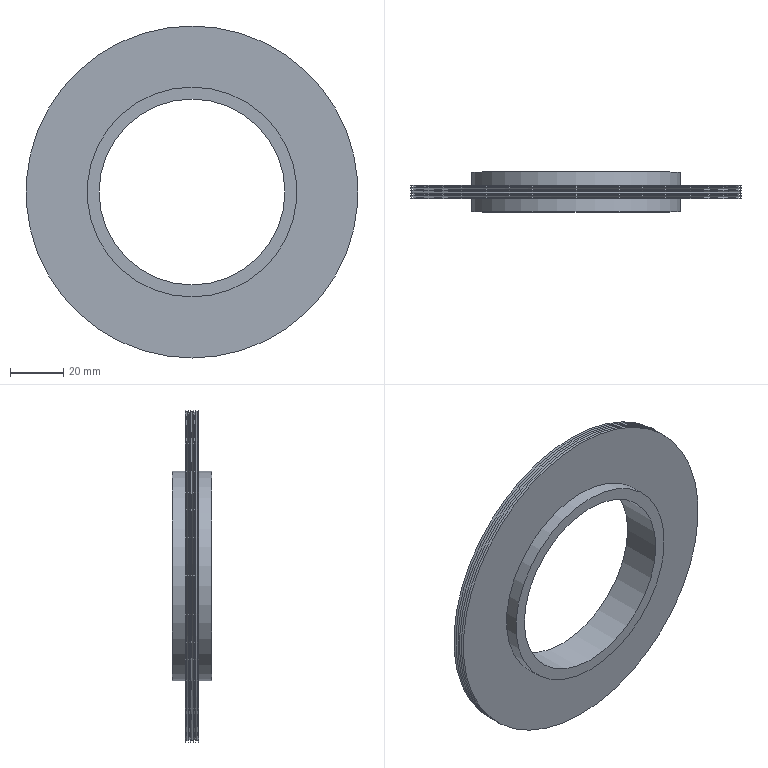Part | NX | 1 solid | 17 faces | box 125 x 15 x 125 mm | volume 51673 mm3 | cone 10 | plane 4 | cylinder 3 | commonest cylinder face diameters 79 x2 70 x1
STEP:
#1=CARTESIAN_POINT('',(0.,18.7,-39.5));
#2=VERTEX_POINT('',#1);
#3=CARTESIAN_POINT('',(0.,18.7,0.));
#4=DIRECTION('',(0.,-1.,0.));
#5=DIRECTION('',(0.,0.,-1.));
#6=AXIS2_PLACEMENT_3D('',#3,#4,#5);
#7=CIRCLE('',#6,39.5);
#8=EDGE_CURVE('',#2,#2,#7,.T.);
#9=ORIENTED_EDGE('',*,*,#8,.T.);
#10=EDGE_LOOP('',(#9));
#11=FACE_BOUND('',#10,.T.);
#12=CARTESIAN_POINT('',(0.,13.7,-39.5));
#13=VERTEX_POINT('',#12);
#14=CARTESIAN_POINT('',(0.,13.7,0.));
#15=DIRECTION('',(0.,-1.,0.));
#16=DIRECTION('',(0.,0.,-1.));
#17=AXIS2_PLACEMENT_3D('',#14,#15,#16);
#18=CIRCLE('',#17,39.5);
#19=EDGE_CURVE('',#13,#13,#18,.T.);
#20=ORIENTED_EDGE('',*,*,#19,.F.);
#21=EDGE_LOOP('',(#20));
#22=FACE_BOUND('',#21,.T.);
#23=CARTESIAN_POINT('',(0.,0.,0.));
#24=DIRECTION('',(0.,-1.,0.));
#25=DIRECTION('',(0.,0.,1.));
#26=AXIS2_PLACEMENT_3D('',#23,#24,#25);
#27=CYLINDRICAL_SURFACE('',#26,39.5);
#28=ADVANCED_FACE('',(#11,#22),#27,.T.);
#29=CARTESIAN_POINT('',(0.,18.7,-35.));
#30=VERTEX_POINT('',#29);
#31=CARTESIAN_POINT('',(0.,18.7,0.));
#32=DIRECTION('',(0.,-1.,0.));
#33=DIRECTION('',(0.,0.,-1.));
#34=AXIS2_PLACEMENT_3D('',#31,#32,#33);
#35=CIRCLE('',#34,35.);
#36=EDGE_CURVE('',#30,#30,#35,.T.);
#37=ORIENTED_EDGE('',*,*,#36,.T.);
#38=EDGE_LOOP('',(#37));
#39=FACE_BOUND('',#38,.T.);
#40=ORIENTED_EDGE('',*,*,#8,.F.);
#41=EDGE_LOOP('',(#40));
#42=FACE_BOUND('',#41,.T.);
#43=CARTESIAN_POINT('',(-39.5,18.7,0.));
#44=DIRECTION('',(0.,1.,0.));
#45=DIRECTION('',(0.,0.,-1.));
#46=AXIS2_PLACEMENT_3D('',#43,#44,#45);
#47=PLANE('',#46);
#48=ADVANCED_FACE('',(#39,#42),#47,.T.);
#49=CARTESIAN_POINT('',(0.,3.7,-35.));
#50=VERTEX_POINT('',#49);
#51=CARTESIAN_POINT('',(0.,3.7,0.));
#52=DIRECTION('',(0.,-1.,0.));
#53=DIRECTION('',(0.,0.,-1.));
#54=AXIS2_PLACEMENT_3D('',#51,#52,#53);
#55=CIRCLE('',#54,35.);
#56=EDGE_CURVE('',#50,#50,#55,.T.);
#57=ORIENTED_EDGE('',*,*,#56,.T.);
#58=EDGE_LOOP('',(#57));
#59=FACE_BOUND('',#58,.T.);
#60=ORIENTED_EDGE('',*,*,#36,.F.);
#61=EDGE_LOOP('',(#60));
#62=FACE_BOUND('',#61,.T.);
#63=CARTESIAN_POINT('',(0.,0.,0.));
#64=DIRECTION('',(0.,-1.,0.));
#65=DIRECTION('',(0.,0.,1.));
#66=AXIS2_PLACEMENT_3D('',#63,#64,#65);
#67=CYLINDRICAL_SURFACE('',#66,35.);
#68=ADVANCED_FACE('',(#59,#62),#67,.F.);
#69=CARTESIAN_POINT('',(0.,3.7,-39.5));
#70=VERTEX_POINT('',#69);
#71=CARTESIAN_POINT('',(0.,3.7,0.));
#72=DIRECTION('',(0.,-1.,0.));
#73=DIRECTION('',(0.,0.,-1.));
#74=AXIS2_PLACEMENT_3D('',#71,#72,#73);
#75=CIRCLE('',#74,39.5);
#76=EDGE_CURVE('',#70,#70,#75,.T.);
#77=ORIENTED_EDGE('',*,*,#76,.T.);
#78=EDGE_LOOP('',(#77));
#79=FACE_BOUND('',#78,.T.);
#80=ORIENTED_EDGE('',*,*,#56,.F.);
#81=EDGE_LOOP('',(#80));
#82=FACE_BOUND('',#81,.T.);
#83=CARTESIAN_POINT('',(-35.,3.7,0.));
#84=DIRECTION('',(0.,-1.,0.));
#85=DIRECTION('',(0.,0.,1.));
#86=AXIS2_PLACEMENT_3D('',#83,#84,#85);
#87=PLANE('',#86);
#88=ADVANCED_FACE('',(#79,#82),#87,.T.);
#89=CARTESIAN_POINT('',(0.,8.7,-39.5));
#90=VERTEX_POINT('',#89);
#91=CARTESIAN_POINT('',(0.,8.7,0.));
#92=DIRECTION('',(0.,-1.,0.));
#93=DIRECTION('',(0.,0.,-1.));
#94=AXIS2_PLACEMENT_3D('',#91,#92,#93);
#95=CIRCLE('',#94,39.5);
#96=EDGE_CURVE('',#90,#90,#95,.T.);
#97=ORIENTED_EDGE('',*,*,#96,.T.);
#98=EDGE_LOOP('',(#97));
#99=FACE_BOUND('',#98,.T.);
#100=ORIENTED_EDGE('',*,*,#76,.F.);
#101=EDGE_LOOP('',(#100));
#102=FACE_BOUND('',#101,.T.);
#103=CARTESIAN_POINT('',(0.,0.,0.));
#104=DIRECTION('',(0.,-1.,0.));
#105=DIRECTION('',(0.,0.,1.));
#106=AXIS2_PLACEMENT_3D('',#103,#104,#105);
#107=CYLINDRICAL_SURFACE('',#106,39.5);
#108=ADVANCED_FACE('',(#99,#102),#107,.T.);
#109=CARTESIAN_POINT('',(0.,8.7,-62.5));
#110=VERTEX_POINT('',#109);
#111=CARTESIAN_POINT('',(0.,8.7,0.));
#112=DIRECTION('',(0.,-1.,0.));
#113=DIRECTION('',(0.,0.,-1.));
#114=AXIS2_PLACEMENT_3D('',#111,#112,#113);
#115=CIRCLE('',#114,62.5);
#116=EDGE_CURVE('',#110,#110,#115,.T.);
#117=ORIENTED_EDGE('',*,*,#116,.T.);
#118=EDGE_LOOP('',(#117));
#119=FACE_BOUND('',#118,.T.);
#120=ORIENTED_EDGE('',*,*,#96,.F.);
#121=EDGE_LOOP('',(#120));
#122=FACE_BOUND('',#121,.T.);
#123=CARTESIAN_POINT('',(-39.5,8.7,0.));
#124=DIRECTION('',(0.,-1.,0.));
#125=DIRECTION('',(0.,0.,1.));
#126=AXIS2_PLACEMENT_3D('',#123,#124,#125);
#127=PLANE('',#126);
#128=ADVANCED_FACE('',(#119,#122),#127,.T.);
#129=CARTESIAN_POINT('',(0.,9.2,-61.5));
#130=VERTEX_POINT('',#129);
#131=CARTESIAN_POINT('',(0.,9.2,0.));
#132=DIRECTION('',(0.,-1.,0.));
#133=DIRECTION('',(0.,0.,-1.));
#134=AXIS2_PLACEMENT_3D('',#131,#132,#133);
#135=CIRCLE('',#134,61.5);
#136=EDGE_CURVE('',#130,#130,#135,.T.);
#137=ORIENTED_EDGE('',*,*,#136,.T.);
#138=EDGE_LOOP('',(#137));
#139=FACE_BOUND('',#138,.T.);
#140=ORIENTED_EDGE('',*,*,#116,.F.);
#141=EDGE_LOOP('',(#140));
#142=FACE_BOUND('',#141,.T.);
#143=CARTESIAN_POINT('',(0.,8.7,0.));
#144=DIRECTION('',(0.,-1.,0.));
#145=DIRECTION('',(0.,0.,1.));
#146=AXIS2_PLACEMENT_3D('',#143,#144,#145);
#147=CONICAL_SURFACE('',#146,62.5,63.435);
#148=ADVANCED_FACE('',(#139,#142),#147,.T.);
#149=CARTESIAN_POINT('',(0.,9.7,-62.5));
#150=VERTEX_POINT('',#149);
#151=CARTESIAN_POINT('',(0.,9.7,0.));
#152=DIRECTION('',(0.,-1.,0.));
#153=DIRECTION('',(0.,0.,-1.));
#154=AXIS2_PLACEMENT_3D('',#151,#152,#153);
#155=CIRCLE('',#154,62.5);
#156=EDGE_CURVE('',#150,#150,#155,.T.);
#157=ORIENTED_EDGE('',*,*,#156,.T.);
#158=EDGE_LOOP('',(#157));
#159=FACE_BOUND('',#158,.T.);
#160=ORIENTED_EDGE('',*,*,#136,.F.);
#161=EDGE_LOOP('',(#160));
#162=FACE_BOUND('',#161,.T.);
#163=CARTESIAN_POINT('',(0.,9.2,0.));
#164=DIRECTION('',(0.,1.,0.));
#165=DIRECTION('',(0.,0.,-1.));
#166=AXIS2_PLACEMENT_3D('',#163,#164,#165);
#167=CONICAL_SURFACE('',#166,61.5,63.435);
#168=ADVANCED_FACE('',(#159,#162),#167,.T.);
#169=CARTESIAN_POINT('',(0.,10.2,-61.5));
#170=VERTEX_POINT('',#169);
#171=CARTESIAN_POINT('',(0.,10.2,0.));
#172=DIRECTION('',(0.,-1.,0.));
#173=DIRECTION('',(0.,0.,-1.));
#174=AXIS2_PLACEMENT_3D('',#171,#172,#173);
#175=CIRCLE('',#174,61.5);
#176=EDGE_CURVE('',#170,#170,#175,.T.);
#177=ORIENTED_EDGE('',*,*,#176,.T.);
#178=EDGE_LOOP('',(#177));
#179=FACE_BOUND('',#178,.T.);
#180=ORIENTED_EDGE('',*,*,#156,.F.);
#181=EDGE_LOOP('',(#180));
#182=FACE_BOUND('',#181,.T.);
#183=CARTESIAN_POINT('',(0.,9.7,0.));
#184=DIRECTION('',(0.,-1.,0.));
#185=DIRECTION('',(0.,0.,1.));
#186=AXIS2_PLACEMENT_3D('',#183,#184,#185);
#187=CONICAL_SURFACE('',#186,62.5,63.435);
#188=ADVANCED_FACE('',(#179,#182),#187,.T.);
#189=CARTESIAN_POINT('',(0.,10.7,-62.5));
#190=VERTEX_POINT('',#189);
#191=CARTESIAN_POINT('',(0.,10.7,0.));
#192=DIRECTION('',(0.,-1.,0.));
#193=DIRECTION('',(0.,0.,-1.));
#194=AXIS2_PLACEMENT_3D('',#191,#192,#193);
#195=CIRCLE('',#194,62.5);
#196=EDGE_CURVE('',#190,#190,#195,.T.);
#197=ORIENTED_EDGE('',*,*,#196,.T.);
#198=EDGE_LOOP('',(#197));
#199=FACE_BOUND('',#198,.T.);
#200=ORIENTED_EDGE('',*,*,#176,.F.);
#201=EDGE_LOOP('',(#200));
#202=FACE_BOUND('',#201,.T.);
#203=CARTESIAN_POINT('',(0.,10.2,0.));
#204=DIRECTION('',(0.,1.,0.));
#205=DIRECTION('',(0.,0.,-1.));
#206=AXIS2_PLACEMENT_3D('',#203,#204,#205);
#207=CONICAL_SURFACE('',#206,61.5,63.435);
#208=ADVANCED_FACE('',(#199,#202),#207,.T.);
#209=CARTESIAN_POINT('',(0.,11.2,-61.5));
#210=VERTEX_POINT('',#209);
#211=CARTESIAN_POINT('',(0.,11.2,0.));
#212=DIRECTION('',(0.,-1.,0.));
#213=DIRECTION('',(0.,0.,-1.));
#214=AXIS2_PLACEMENT_3D('',#211,#212,#213);
#215=CIRCLE('',#214,61.5);
#216=EDGE_CURVE('',#210,#210,#215,.T.);
#217=ORIENTED_EDGE('',*,*,#216,.T.);
#218=EDGE_LOOP('',(#217));
#219=FACE_BOUND('',#218,.T.);
#220=ORIENTED_EDGE('',*,*,#196,.F.);
#221=EDGE_LOOP('',(#220));
#222=FACE_BOUND('',#221,.T.);
#223=CARTESIAN_POINT('',(0.,10.7,0.));
#224=DIRECTION('',(0.,-1.,0.));
#225=DIRECTION('',(0.,0.,1.));
#226=AXIS2_PLACEMENT_3D('',#223,#224,#225);
#227=CONICAL_SURFACE('',#226,62.5,63.435);
#228=ADVANCED_FACE('',(#219,#222),#227,.T.);
#229=CARTESIAN_POINT('',(0.,11.7,-62.5));
#230=VERTEX_POINT('',#229);
#231=CARTESIAN_POINT('',(0.,11.7,0.));
#232=DIRECTION('',(0.,-1.,0.));
#233=DIRECTION('',(0.,0.,-1.));
#234=AXIS2_PLACEMENT_3D('',#231,#232,#233);
#235=CIRCLE('',#234,62.5);
#236=EDGE_CURVE('',#230,#230,#235,.T.);
#237=ORIENTED_EDGE('',*,*,#236,.T.);
#238=EDGE_LOOP('',(#237));
#239=FACE_BOUND('',#238,.T.);
#240=ORIENTED_EDGE('',*,*,#216,.F.);
#241=EDGE_LOOP('',(#240));
#242=FACE_BOUND('',#241,.T.);
#243=CARTESIAN_POINT('',(0.,11.2,0.));
#244=DIRECTION('',(0.,1.,0.));
#245=DIRECTION('',(0.,0.,-1.));
#246=AXIS2_PLACEMENT_3D('',#243,#244,#245);
#247=CONICAL_SURFACE('',#246,61.5,63.435);
#248=ADVANCED_FACE('',(#239,#242),#247,.T.);
#249=CARTESIAN_POINT('',(0.,12.2,-61.5));
#250=VERTEX_POINT('',#249);
#251=CARTESIAN_POINT('',(0.,12.2,0.));
#252=DIRECTION('',(0.,-1.,0.));
#253=DIRECTION('',(0.,0.,-1.));
#254=AXIS2_PLACEMENT_3D('',#251,#252,#253);
#255=CIRCLE('',#254,61.5);
#256=EDGE_CURVE('',#250,#250,#255,.T.);
#257=ORIENTED_EDGE('',*,*,#256,.T.);
#258=EDGE_LOOP('',(#257));
#259=FACE_BOUND('',#258,.T.);
#260=ORIENTED_EDGE('',*,*,#236,.F.);
#261=EDGE_LOOP('',(#260));
#262=FACE_BOUND('',#261,.T.);
#263=CARTESIAN_POINT('',(0.,11.7,0.));
#264=DIRECTION('',(0.,-1.,0.));
#265=DIRECTION('',(0.,0.,1.));
#266=AXIS2_PLACEMENT_3D('',#263,#264,#265);
#267=CONICAL_SURFACE('',#266,62.5,63.435);
#268=ADVANCED_FACE('',(#259,#262),#267,.T.);
#269=CARTESIAN_POINT('',(0.,12.7,-62.5));
#270=VERTEX_POINT('',#269);
#271=CARTESIAN_POINT('',(0.,12.7,0.));
#272=DIRECTION('',(0.,-1.,0.));
#273=DIRECTION('',(0.,0.,-1.));
#274=AXIS2_PLACEMENT_3D('',#271,#272,#273);
#275=CIRCLE('',#274,62.5);
#276=EDGE_CURVE('',#270,#270,#275,.T.);
#277=ORIENTED_EDGE('',*,*,#276,.T.);
#278=EDGE_LOOP('',(#277));
#279=FACE_BOUND('',#278,.T.);
#280=ORIENTED_EDGE('',*,*,#256,.F.);
#281=EDGE_LOOP('',(#280));
#282=FACE_BOUND('',#281,.T.);
#283=CARTESIAN_POINT('',(0.,12.2,0.));
#284=DIRECTION('',(0.,1.,0.));
#285=DIRECTION('',(0.,0.,-1.));
#286=AXIS2_PLACEMENT_3D('',#283,#284,#285);
#287=CONICAL_SURFACE('',#286,61.5,63.435);
#288=ADVANCED_FACE('',(#279,#282),#287,.T.);
#289=CARTESIAN_POINT('',(0.,13.2,-61.5));
#290=VERTEX_POINT('',#289);
#291=CARTESIAN_POINT('',(0.,13.2,0.));
#292=DIRECTION('',(0.,-1.,0.));
#293=DIRECTION('',(0.,0.,-1.));
#294=AXIS2_PLACEMENT_3D('',#291,#292,#293);
#295=CIRCLE('',#294,61.5);
#296=EDGE_CURVE('',#290,#290,#295,.T.);
#297=ORIENTED_EDGE('',*,*,#296,.T.);
#298=EDGE_LOOP('',(#297));
#299=FACE_BOUND('',#298,.T.);
#300=ORIENTED_EDGE('',*,*,#276,.F.);
#301=EDGE_LOOP('',(#300));
#302=FACE_BOUND('',#301,.T.);
#303=CARTESIAN_POINT('',(0.,12.7,0.));
#304=DIRECTION('',(0.,-1.,0.));
#305=DIRECTION('',(0.,0.,1.));
#306=AXIS2_PLACEMENT_3D('',#303,#304,#305);
#307=CONICAL_SURFACE('',#306,62.5,63.435);
#308=ADVANCED_FACE('',(#299,#302),#307,.T.);
#309=CARTESIAN_POINT('',(0.,13.7,-62.5));
#310=VERTEX_POINT('',#309);
#311=CARTESIAN_POINT('',(0.,13.7,0.));
#312=DIRECTION('',(0.,-1.,0.));
#313=DIRECTION('',(0.,0.,-1.));
#314=AXIS2_PLACEMENT_3D('',#311,#312,#313);
#315=CIRCLE('',#314,62.5);
#316=EDGE_CURVE('',#310,#310,#315,.T.);
#317=ORIENTED_EDGE('',*,*,#316,.T.);
#318=EDGE_LOOP('',(#317));
#319=FACE_BOUND('',#318,.T.);
#320=ORIENTED_EDGE('',*,*,#296,.F.);
#321=EDGE_LOOP('',(#320));
#322=FACE_BOUND('',#321,.T.);
#323=CARTESIAN_POINT('',(0.,13.2,0.));
#324=DIRECTION('',(0.,1.,0.));
#325=DIRECTION('',(0.,0.,-1.));
#326=AXIS2_PLACEMENT_3D('',#323,#324,#325);
#327=CONICAL_SURFACE('',#326,61.5,63.435);
#328=ADVANCED_FACE('',(#319,#322),#327,.T.);
#329=ORIENTED_EDGE('',*,*,#19,.T.);
#330=EDGE_LOOP('',(#329));
#331=FACE_BOUND('',#330,.T.);
#332=ORIENTED_EDGE('',*,*,#316,.F.);
#333=EDGE_LOOP('',(#332));
#334=FACE_BOUND('',#333,.T.);
#335=CARTESIAN_POINT('',(-62.5,13.7,0.));
#336=DIRECTION('',(0.,1.,0.));
#337=DIRECTION('',(0.,0.,-1.));
#338=AXIS2_PLACEMENT_3D('',#335,#336,#337);
#339=PLANE('',#338);
#340=ADVANCED_FACE('',(#331,#334),#339,.T.);
#341=CLOSED_SHELL('',(#28,#48,#68,#88,#108,#128,#148,#168,#188,#208,#228,#248,#268,#288,#308,#328,#340));
#342=MANIFOLD_SOLID_BREP('',#341);
#343=(LENGTH_UNIT()NAMED_UNIT(*)SI_UNIT(.MILLI.,.METRE.));
#344=UNCERTAINTY_MEASURE_WITH_UNIT(LENGTH_MEASURE(0.00002),#343,'','');
#345=(NAMED_UNIT(*)PLANE_ANGLE_UNIT()SI_UNIT($,.RADIAN.));
#346=PLANE_ANGLE_MEASURE_WITH_UNIT(PLANE_ANGLE_MEASURE(0.01745),#345);
#347=DIMENSIONAL_EXPONENTS(0.,0.,0.,0.,0.,0.,0.);
#348=(CONVERSION_BASED_UNIT('DEGREE',#346)NAMED_UNIT(#347)PLANE_ANGLE_UNIT());
#349=(NAMED_UNIT(*)SI_UNIT($,.STERADIAN.)SOLID_ANGLE_UNIT());
#350=(GEOMETRIC_REPRESENTATION_CONTEXT(3)GLOBAL_UNCERTAINTY_ASSIGNED_CONTEXT((#344))GLOBAL_UNIT_ASSIGNED_CONTEXT((#343,#348,#349))REPRESENTATION_CONTEXT('',''));
#351=ADVANCED_BREP_SHAPE_REPRESENTATION('',(#342),#350);